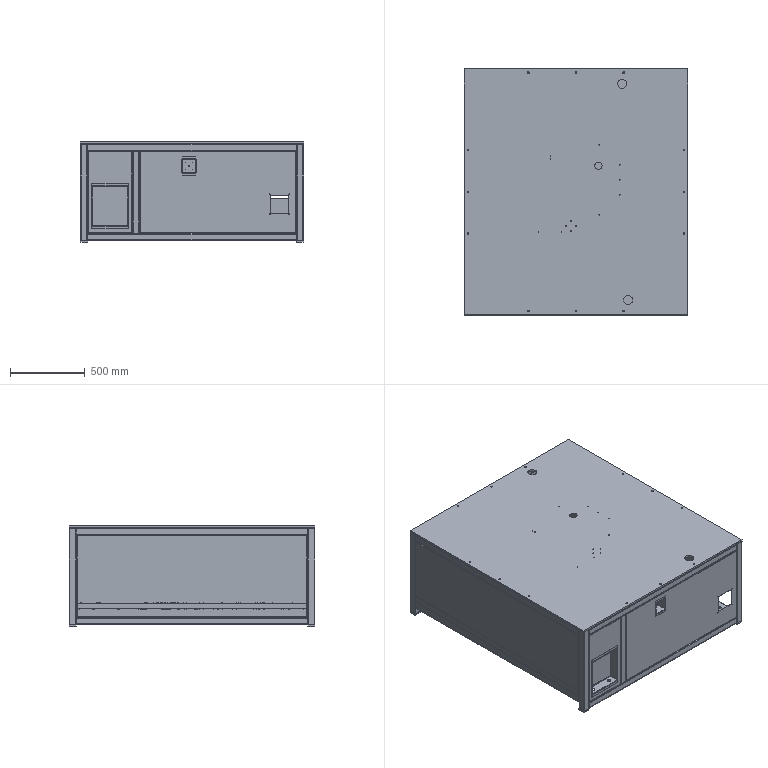Part | SolidWorks | features ICE 14, FlatPattern 12, EdgeFlange 11, HoleWzd 11, SMBaseFlange 9, SheetMetal 9, MirrorSolid 6, MirrorPattern 4, Fillet 3, MoveCopyBody 2, MoveFace 2, WeldCornerFeat 2, 3DProfileFeature 1, Chamfer 1, EndCap 1, WeldMemberFeat 1, WeldmentFeature 1 | 41 solids | 1101 faces | box 1500 x 1650 x 672 mm | volume 49489000 mm3 | plane 557 | cylinder 464 | spline 80 | commonest cylinder face diameters 6 x92 12 x68 6.6 x62 4 x48 5 x44 7 x44